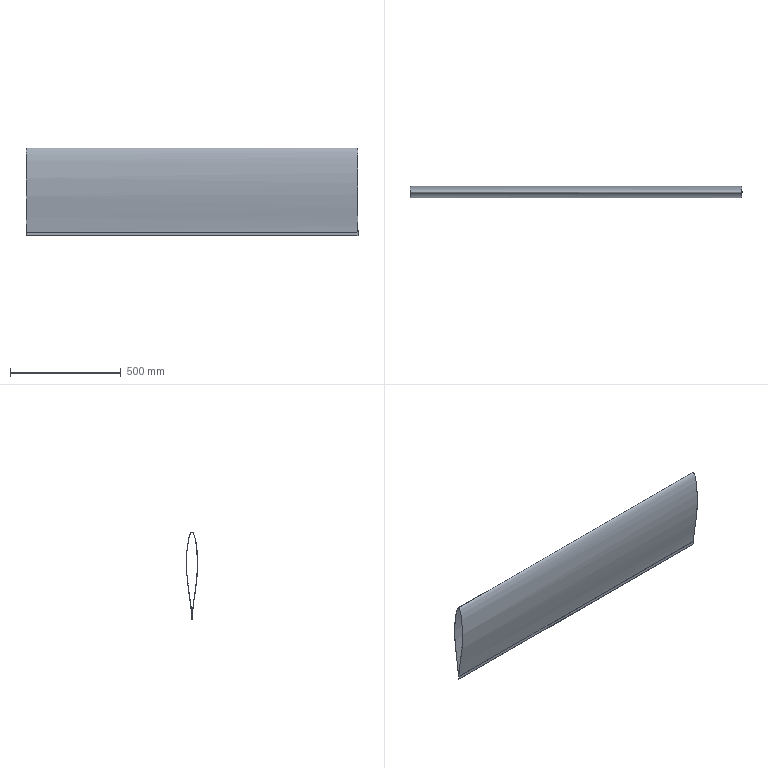Part | SolidWorks | features BaseBody 1 | 1 solid | 10 faces | box 1500 x 51.061 x 395 mm | volume 407991 mm3 | plane 8 | spline 2